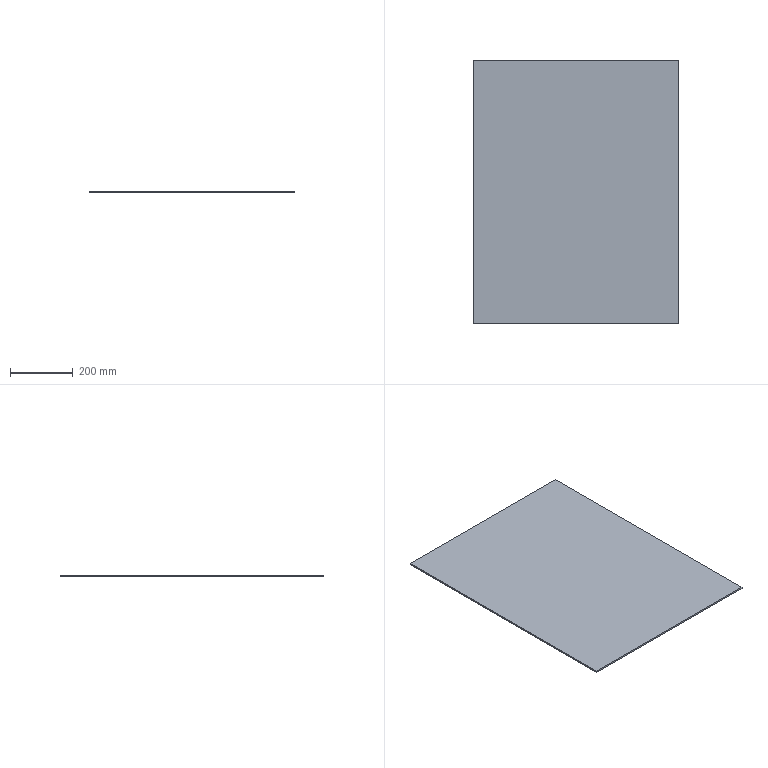Part | SolidWorks | features Extrusion 1, HoleWzd 1 | 1 solid | 6 faces | box 656 x 842 x 5 mm | volume 2761760 mm3 | plane 6
STEP:
#1=CARTESIAN_POINT('',(328.,-421.,0.));
#2=VERTEX_POINT('',#1);
#3=CARTESIAN_POINT('',(328.,421.,0.));
#4=VERTEX_POINT('',#3);
#5=CARTESIAN_POINT('',(328.,421.,0.));
#6=DIRECTION('',(0.,1.,0.));
#7=VECTOR('',#6,1000.);
#8=LINE('',#5,#7);
#9=EDGE_CURVE('',#2,#4,#8,.T.);
#10=ORIENTED_EDGE('',*,*,#9,.T.);
#11=CARTESIAN_POINT('',(328.,421.,5.));
#12=VERTEX_POINT('',#11);
#13=CARTESIAN_POINT('',(328.,421.,5.));
#14=DIRECTION('',(0.,0.,-1.));
#15=VECTOR('',#14,1000.);
#16=LINE('',#13,#15);
#17=EDGE_CURVE('',#12,#4,#16,.T.);
#18=ORIENTED_EDGE('',*,*,#17,.F.);
#19=CARTESIAN_POINT('',(328.,-421.,5.));
#20=VERTEX_POINT('',#19);
#21=CARTESIAN_POINT('',(328.,421.,5.));
#22=DIRECTION('',(0.,1.,0.));
#23=VECTOR('',#22,1000.);
#24=LINE('',#21,#23);
#25=EDGE_CURVE('',#20,#12,#24,.T.);
#26=ORIENTED_EDGE('',*,*,#25,.F.);
#27=CARTESIAN_POINT('',(328.,-421.,5.));
#28=DIRECTION('',(0.,0.,-1.));
#29=VECTOR('',#28,1000.);
#30=LINE('',#27,#29);
#31=EDGE_CURVE('',#20,#2,#30,.T.);
#32=ORIENTED_EDGE('',*,*,#31,.T.);
#33=EDGE_LOOP('',(#10,#18,#26,#32));
#34=FACE_OUTER_BOUND('',#33,.T.);
#35=CARTESIAN_POINT('',(328.,421.,5.));
#36=DIRECTION('',(-1.,0.,0.));
#37=DIRECTION('',(0.,-1.,0.));
#38=AXIS2_PLACEMENT_3D('',#35,#36,#37);
#39=PLANE('',#38);
#40=ADVANCED_FACE('',(#34),#39,.F.);
#41=CARTESIAN_POINT('',(-328.,421.,0.));
#42=VERTEX_POINT('',#41);
#43=CARTESIAN_POINT('',(-328.,421.,0.));
#44=DIRECTION('',(-1.,0.,0.));
#45=VECTOR('',#44,1000.);
#46=LINE('',#43,#45);
#47=EDGE_CURVE('',#4,#42,#46,.T.);
#48=ORIENTED_EDGE('',*,*,#47,.T.);
#49=CARTESIAN_POINT('',(-328.,421.,5.));
#50=VERTEX_POINT('',#49);
#51=CARTESIAN_POINT('',(-328.,421.,5.));
#52=DIRECTION('',(0.,0.,-1.));
#53=VECTOR('',#52,1000.);
#54=LINE('',#51,#53);
#55=EDGE_CURVE('',#50,#42,#54,.T.);
#56=ORIENTED_EDGE('',*,*,#55,.F.);
#57=CARTESIAN_POINT('',(-328.,421.,5.));
#58=DIRECTION('',(-1.,0.,0.));
#59=VECTOR('',#58,1000.);
#60=LINE('',#57,#59);
#61=EDGE_CURVE('',#12,#50,#60,.T.);
#62=ORIENTED_EDGE('',*,*,#61,.F.);
#63=ORIENTED_EDGE('',*,*,#17,.T.);
#64=EDGE_LOOP('',(#48,#56,#62,#63));
#65=FACE_OUTER_BOUND('',#64,.T.);
#66=CARTESIAN_POINT('',(-328.,421.,5.));
#67=DIRECTION('',(0.,-1.,0.));
#68=DIRECTION('',(0.,0.,-1.));
#69=AXIS2_PLACEMENT_3D('',#66,#67,#68);
#70=PLANE('',#69);
#71=ADVANCED_FACE('',(#65),#70,.F.);
#72=CARTESIAN_POINT('',(-328.,-421.,0.));
#73=VERTEX_POINT('',#72);
#74=CARTESIAN_POINT('',(-328.,421.,0.));
#75=DIRECTION('',(0.,-1.,0.));
#76=VECTOR('',#75,1000.);
#77=LINE('',#74,#76);
#78=EDGE_CURVE('',#42,#73,#77,.T.);
#79=ORIENTED_EDGE('',*,*,#78,.T.);
#80=CARTESIAN_POINT('',(-328.,-421.,5.));
#81=VERTEX_POINT('',#80);
#82=CARTESIAN_POINT('',(-328.,-421.,5.));
#83=DIRECTION('',(0.,0.,-1.));
#84=VECTOR('',#83,1000.);
#85=LINE('',#82,#84);
#86=EDGE_CURVE('',#81,#73,#85,.T.);
#87=ORIENTED_EDGE('',*,*,#86,.F.);
#88=CARTESIAN_POINT('',(-328.,421.,5.));
#89=DIRECTION('',(0.,-1.,0.));
#90=VECTOR('',#89,1000.);
#91=LINE('',#88,#90);
#92=EDGE_CURVE('',#50,#81,#91,.T.);
#93=ORIENTED_EDGE('',*,*,#92,.F.);
#94=ORIENTED_EDGE('',*,*,#55,.T.);
#95=EDGE_LOOP('',(#79,#87,#93,#94));
#96=FACE_OUTER_BOUND('',#95,.T.);
#97=CARTESIAN_POINT('',(-328.,421.,5.));
#98=DIRECTION('',(1.,0.,0.));
#99=DIRECTION('',(0.,1.,0.));
#100=AXIS2_PLACEMENT_3D('',#97,#98,#99);
#101=PLANE('',#100);
#102=ADVANCED_FACE('',(#96),#101,.F.);
#103=CARTESIAN_POINT('',(-328.,-421.,0.));
#104=DIRECTION('',(1.,0.,0.));
#105=VECTOR('',#104,1000.);
#106=LINE('',#103,#105);
#107=EDGE_CURVE('',#73,#2,#106,.T.);
#108=ORIENTED_EDGE('',*,*,#107,.T.);
#109=ORIENTED_EDGE('',*,*,#31,.F.);
#110=CARTESIAN_POINT('',(-328.,-421.,5.));
#111=DIRECTION('',(1.,0.,0.));
#112=VECTOR('',#111,1000.);
#113=LINE('',#110,#112);
#114=EDGE_CURVE('',#81,#20,#113,.T.);
#115=ORIENTED_EDGE('',*,*,#114,.F.);
#116=ORIENTED_EDGE('',*,*,#86,.T.);
#117=EDGE_LOOP('',(#108,#109,#115,#116));
#118=FACE_OUTER_BOUND('',#117,.T.);
#119=CARTESIAN_POINT('',(-328.,-421.,5.));
#120=DIRECTION('',(0.,1.,0.));
#121=DIRECTION('',(0.,0.,1.));
#122=AXIS2_PLACEMENT_3D('',#119,#120,#121);
#123=PLANE('',#122);
#124=ADVANCED_FACE('',(#118),#123,.F.);
#125=ORIENTED_EDGE('',*,*,#25,.T.);
#126=ORIENTED_EDGE('',*,*,#61,.T.);
#127=ORIENTED_EDGE('',*,*,#92,.T.);
#128=ORIENTED_EDGE('',*,*,#114,.T.);
#129=EDGE_LOOP('',(#125,#126,#127,#128));
#130=FACE_OUTER_BOUND('',#129,.T.);
#131=CARTESIAN_POINT('',(0.,0.,5.));
#132=DIRECTION('',(0.,0.,1.));
#133=DIRECTION('',(1.,0.,0.));
#134=AXIS2_PLACEMENT_3D('',#131,#132,#133);
#135=PLANE('',#134);
#136=ADVANCED_FACE('',(#130),#135,.T.);
#137=ORIENTED_EDGE('',*,*,#9,.F.);
#138=ORIENTED_EDGE('',*,*,#107,.F.);
#139=ORIENTED_EDGE('',*,*,#78,.F.);
#140=ORIENTED_EDGE('',*,*,#47,.F.);
#141=EDGE_LOOP('',(#137,#138,#139,#140));
#142=FACE_OUTER_BOUND('',#141,.T.);
#143=CARTESIAN_POINT('',(0.,0.,0.));
#144=DIRECTION('',(0.,0.,1.));
#145=DIRECTION('',(1.,0.,0.));
#146=AXIS2_PLACEMENT_3D('',#143,#144,#145);
#147=PLANE('',#146);
#148=ADVANCED_FACE('',(#142),#147,.F.);
#149=CLOSED_SHELL('',(#40,#71,#102,#124,#136,#148));
#150=MANIFOLD_SOLID_BREP('',#149);
#151=CARTESIAN_POINT('',(0.,0.,0.));
#152=DIRECTION('',(0.,0.,1.));
#153=DIRECTION('',(1.,0.,0.));
#154=AXIS2_PLACEMENT_3D('',#151,#152,#153);
#155=(LENGTH_UNIT()NAMED_UNIT(*)SI_UNIT(.MILLI.,.METRE.));
#156=UNCERTAINTY_MEASURE_WITH_UNIT(LENGTH_MEASURE(0.00001),#155,'','');
#157=(NAMED_UNIT(*)PLANE_ANGLE_UNIT()SI_UNIT($,.RADIAN.));
#158=(NAMED_UNIT(*)SI_UNIT($,.STERADIAN.)SOLID_ANGLE_UNIT());
#159=(GEOMETRIC_REPRESENTATION_CONTEXT(3)GLOBAL_UNCERTAINTY_ASSIGNED_CONTEXT((#156))GLOBAL_UNIT_ASSIGNED_CONTEXT((#155,#157,#158))REPRESENTATION_CONTEXT('',''));
#160=ADVANCED_BREP_SHAPE_REPRESENTATION('',(#150,#154),#159);